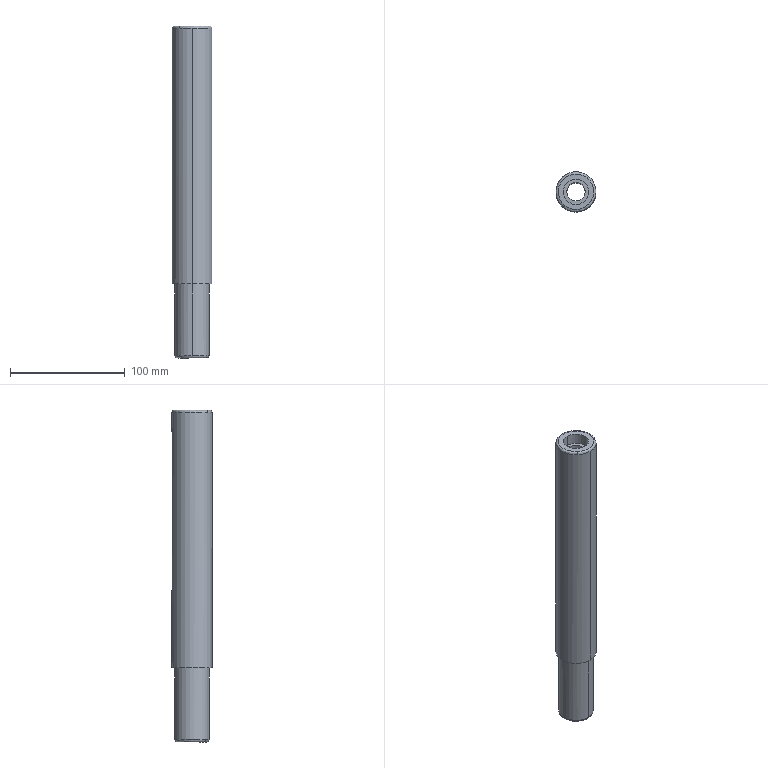Part | SolidWorks | features BaseBody 1 | 1 solid | 35 faces | box 35 x 35 x 289.662 mm | volume 200187 mm3 | cylinder 16 | cone 8 | plane 7 | spline 4 | commonest cylinder face diameters 2.05 x4 4 x2 16 x2 17 x2 22 x2 30 x2
STEP:
#1=CARTESIAN_POINT('',(579.381,24.865,244.432));
#2=VERTEX_POINT('',#1);
#3=CARTESIAN_POINT('',(590.535,55.849,244.432));
#4=VERTEX_POINT('',#3);
#5=CARTESIAN_POINT('',(590.535,38.349,244.432));
#6=DIRECTION('',(0.,0.,-1.));
#7=DIRECTION('',(0.,1.,0.));
#8=AXIS2_PLACEMENT_3D('',#5,#6,#7);
#9=CIRCLE('',#8,17.5);
#10=EDGE_CURVE('',#2,#4,#9,.T.);
#11=ORIENTED_EDGE('',*,*,#10,.F.);
#12=CARTESIAN_POINT('',(580.656,26.406,246.432));
#13=VERTEX_POINT('',#12);
#14=CARTESIAN_POINT('',(580.656,26.406,244.432));
#15=DIRECTION('',(-0.7706,0.6374,0.));
#16=DIRECTION('',(-0.6374,-0.7706,0.));
#17=AXIS2_PLACEMENT_3D('',#14,#15,#16);
#18=CIRCLE('',#17,2.);
#19=EDGE_CURVE('',#2,#13,#18,.T.);
#20=ORIENTED_EDGE('',*,*,#19,.T.);
#21=CARTESIAN_POINT('',(600.414,50.293,246.432));
#22=VERTEX_POINT('',#21);
#23=CARTESIAN_POINT('',(580.656,26.406,246.432));
#24=CARTESIAN_POINT('',(556.769,46.164,246.432));
#25=CARTESIAN_POINT('',(576.527,70.051,246.432));
#26=CARTESIAN_POINT('',(600.414,50.293,246.432));
#27=(BOUNDED_CURVE()B_SPLINE_CURVE(3,(#23,#24,#25,#26),.UNSPECIFIED.,.F.,.F.)B_SPLINE_CURVE_WITH_KNOTS((4,4),(0.,1.),.UNSPECIFIED.)CURVE()GEOMETRIC_REPRESENTATION_ITEM()RATIONAL_B_SPLINE_CURVE((1.,0.3333,0.3333,1.))REPRESENTATION_ITEM(''));
#28=EDGE_CURVE('',#13,#22,#27,.T.);
#29=ORIENTED_EDGE('',*,*,#28,.T.);
#30=CARTESIAN_POINT('',(601.689,51.834,244.432));
#31=VERTEX_POINT('',#30);
#32=CARTESIAN_POINT('',(600.414,50.293,244.432));
#33=DIRECTION('',(0.7706,-0.6374,0.));
#34=DIRECTION('',(0.6374,0.7706,0.));
#35=AXIS2_PLACEMENT_3D('',#32,#33,#34);
#36=CIRCLE('',#35,2.);
#37=EDGE_CURVE('',#31,#22,#36,.T.);
#38=ORIENTED_EDGE('',*,*,#37,.F.);
#39=CARTESIAN_POINT('',(590.535,38.349,244.432));
#40=DIRECTION('',(0.,0.,-1.));
#41=DIRECTION('',(0.,1.,0.));
#42=AXIS2_PLACEMENT_3D('',#39,#40,#41);
#43=CIRCLE('',#42,17.5);
#44=EDGE_CURVE('',#4,#31,#43,.T.);
#45=ORIENTED_EDGE('',*,*,#44,.F.);
#46=EDGE_LOOP('',(#11,#20,#29,#38,#45));
#47=FACE_OUTER_BOUND('',#46,.T.);
#48=CARTESIAN_POINT('',(579.381,24.865,244.432));
#49=CARTESIAN_POINT('',(552.412,47.172,244.432));
#50=CARTESIAN_POINT('',(574.719,74.142,244.432));
#51=CARTESIAN_POINT('',(601.689,51.834,244.432));
#52=CARTESIAN_POINT('',(579.381,24.865,245.604));
#53=CARTESIAN_POINT('',(552.412,47.172,245.604));
#54=CARTESIAN_POINT('',(574.719,74.142,245.604));
#55=CARTESIAN_POINT('',(601.689,51.834,245.604));
#56=CARTESIAN_POINT('',(579.909,25.503,246.432));
#57=CARTESIAN_POINT('',(554.216,46.755,246.432));
#58=CARTESIAN_POINT('',(575.468,72.448,246.432));
#59=CARTESIAN_POINT('',(601.161,51.196,246.432));
#60=CARTESIAN_POINT('',(580.656,26.406,246.432));
#61=CARTESIAN_POINT('',(556.769,46.164,246.432));
#62=CARTESIAN_POINT('',(576.527,70.051,246.432));
#63=CARTESIAN_POINT('',(600.414,50.293,246.432));
#64=(BOUNDED_SURFACE()B_SPLINE_SURFACE(3,3,((#48,#49,#50,#51),(#52,#53,#54,#55),(#56,#57,#58,#59),(#60,#61,#62,#63)),.UNSPECIFIED.,.F.,.F.,.F.)B_SPLINE_SURFACE_WITH_KNOTS((4,4),(4,4),(0.,1.),(0.,1.),.UNSPECIFIED.)GEOMETRIC_REPRESENTATION_ITEM()RATIONAL_B_SPLINE_SURFACE(((1.,0.3333,0.3333,1.),(0.8047,0.2682,0.2682,0.8047),(0.8047,0.2682,0.2682,0.8047),(1.,0.3333,0.3333,1.)))REPRESENTATION_ITEM('')SURFACE());
#65=ADVANCED_FACE('',(#47),#64,.T.);
#66=CARTESIAN_POINT('',(580.975,26.791,-41.23));
#67=VERTEX_POINT('',#66);
#68=CARTESIAN_POINT('',(590.535,23.349,-41.23));
#69=VERTEX_POINT('',#68);
#70=CARTESIAN_POINT('',(590.535,38.349,-41.23));
#71=DIRECTION('',(0.,0.,1.));
#72=DIRECTION('',(0.,1.,0.));
#73=AXIS2_PLACEMENT_3D('',#70,#71,#72);
#74=CIRCLE('',#73,15.);
#75=EDGE_CURVE('',#67,#69,#74,.T.);
#76=ORIENTED_EDGE('',*,*,#75,.F.);
#77=CARTESIAN_POINT('',(582.249,28.332,-43.23));
#78=VERTEX_POINT('',#77);
#79=CARTESIAN_POINT('',(582.249,28.332,-41.23));
#80=DIRECTION('',(0.7706,-0.6374,0.));
#81=DIRECTION('',(-0.6374,-0.7706,0.));
#82=AXIS2_PLACEMENT_3D('',#79,#80,#81);
#83=CIRCLE('',#82,2.);
#84=EDGE_CURVE('',#67,#78,#83,.T.);
#85=ORIENTED_EDGE('',*,*,#84,.T.);
#86=CARTESIAN_POINT('',(598.821,48.367,-43.23));
#87=VERTEX_POINT('',#86);
#88=CARTESIAN_POINT('',(582.249,28.332,-43.23));
#89=CARTESIAN_POINT('',(602.284,11.761,-43.23));
#90=CARTESIAN_POINT('',(618.856,31.795,-43.23));
#91=CARTESIAN_POINT('',(598.821,48.367,-43.23));
#92=(BOUNDED_CURVE()B_SPLINE_CURVE(3,(#88,#89,#90,#91),.UNSPECIFIED.,.F.,.T.)B_SPLINE_CURVE_WITH_KNOTS((4,4),(0.,1.),.UNSPECIFIED.)CURVE()GEOMETRIC_REPRESENTATION_ITEM()RATIONAL_B_SPLINE_CURVE((1.,0.3333,0.3333,1.))REPRESENTATION_ITEM(''));
#93=EDGE_CURVE('',#78,#87,#92,.T.);
#94=ORIENTED_EDGE('',*,*,#93,.T.);
#95=CARTESIAN_POINT('',(600.096,49.908,-41.23));
#96=VERTEX_POINT('',#95);
#97=CARTESIAN_POINT('',(598.821,48.367,-41.23));
#98=DIRECTION('',(-0.7706,0.6374,0.));
#99=DIRECTION('',(0.6374,0.7706,0.));
#100=AXIS2_PLACEMENT_3D('',#97,#98,#99);
#101=CIRCLE('',#100,2.);
#102=EDGE_CURVE('',#96,#87,#101,.T.);
#103=ORIENTED_EDGE('',*,*,#102,.F.);
#104=CARTESIAN_POINT('',(590.535,38.349,-41.23));
#105=DIRECTION('',(0.,0.,1.));
#106=DIRECTION('',(0.,1.,0.));
#107=AXIS2_PLACEMENT_3D('',#104,#105,#106);
#108=CIRCLE('',#107,15.);
#109=EDGE_CURVE('',#69,#96,#108,.T.);
#110=ORIENTED_EDGE('',*,*,#109,.F.);
#111=EDGE_LOOP('',(#76,#85,#94,#103,#110));
#112=FACE_OUTER_BOUND('',#111,.T.);
#113=CARTESIAN_POINT('',(580.975,26.791,-41.23));
#114=CARTESIAN_POINT('',(604.092,7.67,-41.23));
#115=CARTESIAN_POINT('',(623.212,30.787,-41.23));
#116=CARTESIAN_POINT('',(600.096,49.908,-41.23));
#117=CARTESIAN_POINT('',(580.975,26.791,-42.401));
#118=CARTESIAN_POINT('',(604.092,7.67,-42.401));
#119=CARTESIAN_POINT('',(623.212,30.787,-42.401));
#120=CARTESIAN_POINT('',(600.096,49.908,-42.401));
#121=CARTESIAN_POINT('',(581.503,27.429,-43.23));
#122=CARTESIAN_POINT('',(603.343,9.364,-43.23));
#123=CARTESIAN_POINT('',(621.408,31.205,-43.23));
#124=CARTESIAN_POINT('',(599.568,49.27,-43.23));
#125=CARTESIAN_POINT('',(582.249,28.332,-43.23));
#126=CARTESIAN_POINT('',(602.284,11.761,-43.23));
#127=CARTESIAN_POINT('',(618.856,31.795,-43.23));
#128=CARTESIAN_POINT('',(598.821,48.367,-43.23));
#129=(BOUNDED_SURFACE()B_SPLINE_SURFACE(3,3,((#113,#114,#115,#116),(#117,#118,#119,#120),(#121,#122,#123,#124),(#125,#126,#127,#128)),.UNSPECIFIED.,.F.,.F.,.F.)B_SPLINE_SURFACE_WITH_KNOTS((4,4),(4,4),(0.,1.),(0.,1.),.UNSPECIFIED.)GEOMETRIC_REPRESENTATION_ITEM()RATIONAL_B_SPLINE_SURFACE(((1.,0.3333,0.3333,1.),(0.8047,0.2682,0.2682,0.8047),(0.8047,0.2682,0.2682,0.8047),(1.,0.3333,0.3333,1.)))REPRESENTATION_ITEM('')SURFACE());
#130=ADVANCED_FACE('',(#112),#129,.T.);
#131=ORIENTED_EDGE('',*,*,#44,.T.);
#132=CARTESIAN_POINT('',(590.535,20.849,244.432));
#133=VERTEX_POINT('',#132);
#134=CARTESIAN_POINT('',(590.535,38.349,244.432));
#135=DIRECTION('',(0.,0.,-1.));
#136=DIRECTION('',(0.,1.,0.));
#137=AXIS2_PLACEMENT_3D('',#134,#135,#136);
#138=CIRCLE('',#137,17.5);
#139=EDGE_CURVE('',#31,#133,#138,.T.);
#140=ORIENTED_EDGE('',*,*,#139,.T.);
#141=CARTESIAN_POINT('',(590.535,20.849,21.432));
#142=VERTEX_POINT('',#141);
#143=CARTESIAN_POINT('',(590.535,20.849,246.432));
#144=DIRECTION('',(0.,0.,-1.));
#145=VECTOR('',#144,1000.);
#146=LINE('',#143,#145);
#147=EDGE_CURVE('',#133,#142,#146,.T.);
#148=ORIENTED_EDGE('',*,*,#147,.T.);
#149=CARTESIAN_POINT('',(590.535,55.849,21.432));
#150=VERTEX_POINT('',#149);
#151=CARTESIAN_POINT('',(590.535,38.349,21.432));
#152=DIRECTION('',(0.,0.,1.));
#153=DIRECTION('',(0.,1.,0.));
#154=AXIS2_PLACEMENT_3D('',#151,#152,#153);
#155=CIRCLE('',#154,17.5);
#156=EDGE_CURVE('',#142,#150,#155,.T.);
#157=ORIENTED_EDGE('',*,*,#156,.T.);
#158=CARTESIAN_POINT('',(590.535,55.849,88.433));
#159=VERTEX_POINT('',#158);
#160=CARTESIAN_POINT('',(590.535,55.849,246.432));
#161=DIRECTION('',(0.,0.,-1.));
#162=VECTOR('',#161,1000.);
#163=LINE('',#160,#162);
#164=EDGE_CURVE('',#159,#150,#163,.T.);
#165=ORIENTED_EDGE('',*,*,#164,.F.);
#166=CARTESIAN_POINT('',(592.459,55.743,90.432));
#167=VERTEX_POINT('',#166);
#168=CARTESIAN_POINT('',(590.535,55.849,88.433));
#169=CARTESIAN_POINT('',(590.663,55.849,88.438));
#170=CARTESIAN_POINT('',(590.789,55.848,88.455));
#171=CARTESIAN_POINT('',(591.037,55.843,88.513));
#172=CARTESIAN_POINT('',(591.161,55.839,88.555));
#173=CARTESIAN_POINT('',(591.393,55.829,88.659));
#174=CARTESIAN_POINT('',(591.504,55.823,88.722));
#175=CARTESIAN_POINT('',(591.713,55.81,88.868));
#176=CARTESIAN_POINT('',(591.811,55.803,88.953));
#177=CARTESIAN_POINT('',(592.076,55.782,89.227));
#178=CARTESIAN_POINT('',(592.218,55.769,89.446));
#179=CARTESIAN_POINT('',(592.409,55.749,89.918));
#180=CARTESIAN_POINT('',(592.459,55.743,90.174));
#181=CARTESIAN_POINT('',(592.459,55.743,90.432));
#182=B_SPLINE_CURVE_WITH_KNOTS('',3,(#168,#169,#170,#171,#172,#173,#174,#175,#176,#177,#178,#179,#180,#181),.UNSPECIFIED.,.F.,.F.,(4,2,2,2,2,2,4),(0.00007532,0.0004568,0.0008382,0.00122,0.001601,0.002364,0.003127),.UNSPECIFIED.);
#183=EDGE_CURVE('',#159,#167,#182,.T.);
#184=ORIENTED_EDGE('',*,*,#183,.T.);
#185=CARTESIAN_POINT('',(592.459,55.743,226.432));
#186=VERTEX_POINT('',#185);
#187=CARTESIAN_POINT('',(592.459,55.743,246.432));
#188=DIRECTION('',(0.,0.,1.));
#189=VECTOR('',#188,1000.);
#190=LINE('',#187,#189);
#191=EDGE_CURVE('',#167,#186,#190,.T.);
#192=ORIENTED_EDGE('',*,*,#191,.T.);
#193=CARTESIAN_POINT('',(590.535,55.849,228.431));
#194=VERTEX_POINT('',#193);
#195=CARTESIAN_POINT('',(592.459,55.743,226.432));
#196=CARTESIAN_POINT('',(592.459,55.743,226.561));
#197=CARTESIAN_POINT('',(592.447,55.745,226.688));
#198=CARTESIAN_POINT('',(592.399,55.75,226.937));
#199=CARTESIAN_POINT('',(592.362,55.754,227.061));
#200=CARTESIAN_POINT('',(592.266,55.764,227.299));
#201=CARTESIAN_POINT('',(592.208,55.769,227.412));
#202=CARTESIAN_POINT('',(592.069,55.782,227.625));
#203=CARTESIAN_POINT('',(591.989,55.789,227.727));
#204=CARTESIAN_POINT('',(591.812,55.803,227.911));
#205=CARTESIAN_POINT('',(591.716,55.81,227.993));
#206=CARTESIAN_POINT('',(591.507,55.823,228.141));
#207=CARTESIAN_POINT('',(591.394,55.829,228.204));
#208=CARTESIAN_POINT('',(591.046,55.844,228.361));
#209=CARTESIAN_POINT('',(590.792,55.849,228.421));
#210=CARTESIAN_POINT('',(590.535,55.849,228.431));
#211=B_SPLINE_CURVE_WITH_KNOTS('',3,(#195,#196,#197,#198,#199,#200,#201,#202,#203,#204,#205,#206,#207,#208,#209,#210),.UNSPECIFIED.,.F.,.F.,(4,2,2,2,2,2,2,4),(-0.003127,-0.002745,-0.002364,-0.001982,-0.001601,-0.00122,-0.0008381,-0.00007524),.UNSPECIFIED.);
#212=EDGE_CURVE('',#186,#194,#211,.T.);
#213=ORIENTED_EDGE('',*,*,#212,.T.);
#214=CARTESIAN_POINT('',(590.535,55.849,246.432));
#215=DIRECTION('',(0.,0.,-1.));
#216=VECTOR('',#215,1000.);
#217=LINE('',#214,#216);
#218=EDGE_CURVE('',#4,#194,#217,.T.);
#219=ORIENTED_EDGE('',*,*,#218,.F.);
#220=EDGE_LOOP('',(#131,#140,#148,#157,#165,#184,#192,#213,#219));
#221=FACE_OUTER_BOUND('',#220,.T.);
#222=CARTESIAN_POINT('',(590.535,38.349,246.432));
#223=DIRECTION('',(0.,0.,-1.));
#224=DIRECTION('',(0.,1.,0.));
#225=AXIS2_PLACEMENT_3D('',#222,#223,#224);
#226=CYLINDRICAL_SURFACE('',#225,17.5);
#227=ADVANCED_FACE('',(#221),#226,.T.);
#228=CARTESIAN_POINT('',(590.535,23.349,21.432));
#229=VERTEX_POINT('',#228);
#230=CARTESIAN_POINT('',(590.535,53.349,21.432));
#231=VERTEX_POINT('',#230);
#232=CARTESIAN_POINT('',(590.535,38.349,21.432));
#233=DIRECTION('',(0.,0.,1.));
#234=DIRECTION('',(0.,1.,0.));
#235=AXIS2_PLACEMENT_3D('',#232,#233,#234);
#236=CIRCLE('',#235,15.);
#237=EDGE_CURVE('',#229,#231,#236,.T.);
#238=ORIENTED_EDGE('',*,*,#237,.F.);
#239=CARTESIAN_POINT('',(590.535,23.349,21.432));
#240=DIRECTION('',(0.,0.,-1.));
#241=VECTOR('',#240,1000.);
#242=LINE('',#239,#241);
#243=EDGE_CURVE('',#229,#69,#242,.T.);
#244=ORIENTED_EDGE('',*,*,#243,.T.);
#245=ORIENTED_EDGE('',*,*,#109,.T.);
#246=CARTESIAN_POINT('',(590.535,53.349,-41.23));
#247=VERTEX_POINT('',#246);
#248=CARTESIAN_POINT('',(590.535,38.349,-41.23));
#249=DIRECTION('',(0.,0.,1.));
#250=DIRECTION('',(0.,1.,0.));
#251=AXIS2_PLACEMENT_3D('',#248,#249,#250);
#252=CIRCLE('',#251,15.);
#253=EDGE_CURVE('',#96,#247,#252,.T.);
#254=ORIENTED_EDGE('',*,*,#253,.T.);
#255=CARTESIAN_POINT('',(590.535,53.349,21.432));
#256=DIRECTION('',(0.,0.,-1.));
#257=VECTOR('',#256,1000.);
#258=LINE('',#255,#257);
#259=EDGE_CURVE('',#231,#247,#258,.T.);
#260=ORIENTED_EDGE('',*,*,#259,.F.);
#261=EDGE_LOOP('',(#238,#244,#245,#254,#260));
#262=FACE_OUTER_BOUND('',#261,.T.);
#263=CARTESIAN_POINT('',(590.535,38.349,21.432));
#264=DIRECTION('',(0.,0.,-1.));
#265=DIRECTION('',(0.,1.,0.));
#266=AXIS2_PLACEMENT_3D('',#263,#264,#265);
#267=CYLINDRICAL_SURFACE('',#266,15.);
#268=ADVANCED_FACE('',(#262),#267,.T.);
#269=CARTESIAN_POINT('',(590.535,49.349,246.432));
#270=VERTEX_POINT('',#269);
#271=CARTESIAN_POINT('',(590.535,27.349,246.432));
#272=VERTEX_POINT('',#271);
#273=CARTESIAN_POINT('',(590.535,38.349,246.432));
#274=DIRECTION('',(0.,0.,1.));
#275=DIRECTION('',(0.,1.,0.));
#276=AXIS2_PLACEMENT_3D('',#273,#274,#275);
#277=CIRCLE('',#276,11.);
#278=EDGE_CURVE('',#270,#272,#277,.T.);
#279=ORIENTED_EDGE('',*,*,#278,.T.);
#280=CARTESIAN_POINT('',(590.535,27.349,236.432));
#281=VERTEX_POINT('',#280);
#282=CARTESIAN_POINT('',(590.535,27.349,246.432));
#283=DIRECTION('',(0.,0.,-1.));
#284=VECTOR('',#283,1000.);
#285=LINE('',#282,#284);
#286=EDGE_CURVE('',#272,#281,#285,.T.);
#287=ORIENTED_EDGE('',*,*,#286,.T.);
#288=CARTESIAN_POINT('',(590.535,49.349,236.432));
#289=VERTEX_POINT('',#288);
#290=CARTESIAN_POINT('',(590.535,38.349,236.432));
#291=DIRECTION('',(0.,0.,1.));
#292=DIRECTION('',(0.,1.,0.));
#293=AXIS2_PLACEMENT_3D('',#290,#291,#292);
#294=CIRCLE('',#293,11.);
#295=EDGE_CURVE('',#289,#281,#294,.T.);
#296=ORIENTED_EDGE('',*,*,#295,.F.);
#297=CARTESIAN_POINT('',(590.535,49.349,246.432));
#298=DIRECTION('',(0.,0.,-1.));
#299=VECTOR('',#298,1000.);
#300=LINE('',#297,#299);
#301=EDGE_CURVE('',#270,#289,#300,.T.);
#302=ORIENTED_EDGE('',*,*,#301,.F.);
#303=EDGE_LOOP('',(#279,#287,#296,#302));
#304=FACE_OUTER_BOUND('',#303,.T.);
#305=CARTESIAN_POINT('',(590.535,38.349,246.432));
#306=DIRECTION('',(0.,0.,-1.));
#307=DIRECTION('',(0.,1.,0.));
#308=AXIS2_PLACEMENT_3D('',#305,#306,#307);
#309=CYLINDRICAL_SURFACE('',#308,11.);
#310=ADVANCED_FACE('',(#304),#309,.F.);
#311=CARTESIAN_POINT('',(591.494,53.654,226.432));
#312=VERTEX_POINT('',#311);
#313=CARTESIAN_POINT('',(589.444,53.645,226.432));
#314=VERTEX_POINT('',#313);
#315=CARTESIAN_POINT('',(590.469,53.649,226.432));
#316=DIRECTION('',(-0.004352,1.,0.));
#317=DIRECTION('',(-1.,-0.004352,0.));
#318=AXIS2_PLACEMENT_3D('',#315,#316,#317);
#319=CIRCLE('',#318,1.025);
#320=EDGE_CURVE('',#312,#314,#319,.T.);
#321=ORIENTED_EDGE('',*,*,#320,.F.);
#322=CARTESIAN_POINT('',(591.693,53.855,226.432));
#323=VERTEX_POINT('',#322);
#324=CARTESIAN_POINT('',(591.693,53.855,226.432));
#325=DIRECTION('',(0.704,0.7102,0.));
#326=VECTOR('',#325,1000.);
#327=LINE('',#324,#326);
#328=EDGE_CURVE('',#312,#323,#327,.T.);
#329=ORIENTED_EDGE('',*,*,#328,.T.);
#330=CARTESIAN_POINT('',(589.243,53.844,226.432));
#331=VERTEX_POINT('',#330);
#332=CARTESIAN_POINT('',(590.468,53.849,226.432));
#333=DIRECTION('',(-0.004352,1.,0.));
#334=DIRECTION('',(-1.,-0.004352,0.));
#335=AXIS2_PLACEMENT_3D('',#332,#333,#334);
#336=CIRCLE('',#335,1.225);
#337=EDGE_CURVE('',#323,#331,#336,.T.);
#338=ORIENTED_EDGE('',*,*,#337,.T.);
#339=CARTESIAN_POINT('',(589.243,53.844,226.432));
#340=DIRECTION('',(-0.7102,0.704,0.));
#341=VECTOR('',#340,1000.);
#342=LINE('',#339,#341);
#343=EDGE_CURVE('',#314,#331,#342,.T.);
#344=ORIENTED_EDGE('',*,*,#343,.F.);
#345=EDGE_LOOP('',(#321,#329,#338,#344));
#346=FACE_OUTER_BOUND('',#345,.T.);
#347=CARTESIAN_POINT('',(590.468,53.849,226.432));
#348=DIRECTION('',(-0.004352,1.,0.));
#349=DIRECTION('',(-1.,-0.004352,0.));
#350=AXIS2_PLACEMENT_3D('',#347,#348,#349);
#351=CONICAL_SURFACE('',#350,1.225,0.7854);
#352=ADVANCED_FACE('',(#346),#351,.F.);
#353=CARTESIAN_POINT('',(591.494,53.654,90.432));
#354=VERTEX_POINT('',#353);
#355=CARTESIAN_POINT('',(589.444,53.645,90.432));
#356=VERTEX_POINT('',#355);
#357=CARTESIAN_POINT('',(590.469,53.649,90.432));
#358=DIRECTION('',(-0.004352,1.,0.));
#359=DIRECTION('',(-1.,-0.004352,0.));
#360=AXIS2_PLACEMENT_3D('',#357,#358,#359);
#361=CIRCLE('',#360,1.025);
#362=EDGE_CURVE('',#354,#356,#361,.T.);
#363=ORIENTED_EDGE('',*,*,#362,.F.);
#364=CARTESIAN_POINT('',(591.693,53.855,90.432));
#365=VERTEX_POINT('',#364);
#366=CARTESIAN_POINT('',(591.693,53.855,90.432));
#367=DIRECTION('',(0.704,0.7102,0.));
#368=VECTOR('',#367,1000.);
#369=LINE('',#366,#368);
#370=EDGE_CURVE('',#354,#365,#369,.T.);
#371=ORIENTED_EDGE('',*,*,#370,.T.);
#372=CARTESIAN_POINT('',(589.243,53.844,90.432));
#373=VERTEX_POINT('',#372);
#374=CARTESIAN_POINT('',(590.468,53.849,90.432));
#375=DIRECTION('',(-0.004352,1.,0.));
#376=DIRECTION('',(-1.,-0.004352,0.));
#377=AXIS2_PLACEMENT_3D('',#374,#375,#376);
#378=CIRCLE('',#377,1.225);
#379=EDGE_CURVE('',#365,#373,#378,.T.);
#380=ORIENTED_EDGE('',*,*,#379,.T.);
#381=CARTESIAN_POINT('',(589.243,53.844,90.432));
#382=DIRECTION('',(-0.7102,0.704,0.));
#383=VECTOR('',#382,1000.);
#384=LINE('',#381,#383);
#385=EDGE_CURVE('',#356,#373,#384,.T.);
#386=ORIENTED_EDGE('',*,*,#385,.F.);
#387=EDGE_LOOP('',(#363,#371,#380,#386));
#388=FACE_OUTER_BOUND('',#387,.T.);
#389=CARTESIAN_POINT('',(590.468,53.849,90.432));
#390=DIRECTION('',(-0.004352,1.,0.));
#391=DIRECTION('',(-1.,-0.004352,0.));
#392=AXIS2_PLACEMENT_3D('',#389,#390,#391);
#393=CONICAL_SURFACE('',#392,1.225,0.7854);
#394=ADVANCED_FACE('',(#388),#393,.F.);
#395=CARTESIAN_POINT('',(590.535,46.349,-17.734));
#396=VERTEX_POINT('',#395);
#397=CARTESIAN_POINT('',(590.535,30.349,-17.734));
#398=VERTEX_POINT('',#397);
#399=CARTESIAN_POINT('',(590.535,38.349,-17.734));
#400=DIRECTION('',(0.,0.,1.));
#401=DIRECTION('',(0.,-1.,0.));
#402=AXIS2_PLACEMENT_3D('',#399,#400,#401);
#403=CIRCLE('',#402,8.);
#404=EDGE_CURVE('',#396,#398,#403,.T.);
#405=ORIENTED_EDGE('',*,*,#404,.F.);
#406=CARTESIAN_POINT('',(590.535,46.349,89.408));
#407=VERTEX_POINT('',#406);
#408=CARTESIAN_POINT('',(590.535,46.349,-43.568));
#409=DIRECTION('',(0.,0.,1.));
#410=VECTOR('',#409,1000.);
#411=LINE('',#408,#410);
#412=EDGE_CURVE('',#396,#407,#411,.T.);
#413=ORIENTED_EDGE('',*,*,#412,.T.);
#414=CARTESIAN_POINT('',(589.476,46.279,90.432));
#415=VERTEX_POINT('',#414);
#416=CARTESIAN_POINT('',(589.476,46.279,90.432));
#417=CARTESIAN_POINT('',(589.476,46.279,90.293));
#418=CARTESIAN_POINT('',(589.504,46.283,90.157));
#419=CARTESIAN_POINT('',(589.611,46.296,89.905));
#420=CARTESIAN_POINT('',(589.69,46.305,89.79));
#421=CARTESIAN_POINT('',(589.886,46.324,89.6));
#422=CARTESIAN_POINT('',(590.005,46.333,89.524));
#423=CARTESIAN_POINT('',(590.26,46.346,89.426));
#424=CARTESIAN_POINT('',(590.398,46.349,89.403));
#425=CARTESIAN_POINT('',(590.535,46.349,89.408));
#426=B_SPLINE_CURVE_WITH_KNOTS('',3,(#416,#417,#418,#419,#420,#421,#422,#423,#424,#425),.UNSPECIFIED.,.F.,.F.,(4,2,2,2,4),(0.,0.0004098,0.0008195,0.001229,0.001639),.UNSPECIFIED.);
#427=EDGE_CURVE('',#415,#407,#426,.T.);
#428=ORIENTED_EDGE('',*,*,#427,.F.);
#429=CARTESIAN_POINT('',(590.535,46.349,91.456));
#430=VERTEX_POINT('',#429);
#431=CARTESIAN_POINT('',(590.535,46.349,91.456));
#432=CARTESIAN_POINT('',(590.399,46.349,91.461));
#433=CARTESIAN_POINT('',(590.26,46.346,91.438));
#434=CARTESIAN_POINT('',(590.005,46.333,91.34));
#435=CARTESIAN_POINT('',(589.888,46.324,91.265));
#436=CARTESIAN_POINT('',(589.59,46.296,90.978));
#437=CARTESIAN_POINT('',(589.476,46.279,90.709));
#438=CARTESIAN_POINT('',(589.476,46.279,90.432));
#439=B_SPLINE_CURVE_WITH_KNOTS('',3,(#431,#432,#433,#434,#435,#436,#437,#438),.UNSPECIFIED.,.F.,.F.,(4,2,2,4),(0.004777,0.005186,0.005596,0.006414),.UNSPECIFIED.);
#440=EDGE_CURVE('',#430,#415,#439,.T.);
#441=ORIENTED_EDGE('',*,*,#440,.F.);
#442=CARTESIAN_POINT('',(590.535,46.349,225.408));
#443=VERTEX_POINT('',#442);
#444=CARTESIAN_POINT('',(590.535,46.349,-43.568));
#445=DIRECTION('',(0.,0.,1.));
#446=VECTOR('',#445,1000.);
#447=LINE('',#444,#446);
#448=EDGE_CURVE('',#430,#443,#447,.T.);
#449=ORIENTED_EDGE('',*,*,#448,.T.);
#450=CARTESIAN_POINT('',(589.476,46.279,226.432));
#451=VERTEX_POINT('',#450);
#452=CARTESIAN_POINT('',(589.476,46.279,226.432));
#453=CARTESIAN_POINT('',(589.476,46.279,226.293));
#454=CARTESIAN_POINT('',(589.504,46.283,226.157));
#455=CARTESIAN_POINT('',(589.611,46.296,225.905));
#456=CARTESIAN_POINT('',(589.69,46.305,225.79));
#457=CARTESIAN_POINT('',(589.886,46.324,225.6));
#458=CARTESIAN_POINT('',(590.005,46.333,225.524));
#459=CARTESIAN_POINT('',(590.26,46.346,225.426));
#460=CARTESIAN_POINT('',(590.398,46.349,225.403));
#461=CARTESIAN_POINT('',(590.535,46.349,225.408));
#462=B_SPLINE_CURVE_WITH_KNOTS('',3,(#452,#453,#454,#455,#456,#457,#458,#459,#460,#461),.UNSPECIFIED.,.F.,.F.,(4,2,2,2,4),(0.,0.0004098,0.0008195,0.001229,0.001639),.UNSPECIFIED.);
#463=EDGE_CURVE('',#451,#443,#462,.T.);
#464=ORIENTED_EDGE('',*,*,#463,.F.);
#465=CARTESIAN_POINT('',(590.535,46.349,227.456));
#466=VERTEX_POINT('',#465);
#467=CARTESIAN_POINT('',(590.535,46.349,227.456));
#468=CARTESIAN_POINT('',(590.399,46.349,227.461));
#469=CARTESIAN_POINT('',(590.26,46.346,227.438));
#470=CARTESIAN_POINT('',(590.005,46.333,227.34));
#471=CARTESIAN_POINT('',(589.888,46.324,227.265));
#472=CARTESIAN_POINT('',(589.59,46.296,226.978));
#473=CARTESIAN_POINT('',(589.476,46.279,226.709));
#474=CARTESIAN_POINT('',(589.476,46.279,226.432));
#475=B_SPLINE_CURVE_WITH_KNOTS('',3,(#467,#468,#469,#470,#471,#472,#473,#474),.UNSPECIFIED.,.F.,.F.,(4,2,2,4),(0.004777,0.005186,0.005596,0.006414),.UNSPECIFIED.);
#476=EDGE_CURVE('',#466,#451,#475,.T.);
#477=ORIENTED_EDGE('',*,*,#476,.F.);
#478=CARTESIAN_POINT('',(590.535,46.349,236.432));
#479=VERTEX_POINT('',#478);
#480=CARTESIAN_POINT('',(590.535,46.349,-43.568));
#481=DIRECTION('',(0.,0.,1.));
#482=VECTOR('',#481,1000.);
#483=LINE('',#480,#482);
#484=EDGE_CURVE('',#466,#479,#483,.T.);
#485=ORIENTED_EDGE('',*,*,#484,.T.);
#486=CARTESIAN_POINT('',(590.535,30.349,236.432));
#487=VERTEX_POINT('',#486);
#488=CARTESIAN_POINT('',(590.535,38.349,236.432));
#489=DIRECTION('',(0.,0.,1.));
#490=DIRECTION('',(0.,-1.,0.));
#491=AXIS2_PLACEMENT_3D('',#488,#489,#490);
#492=CIRCLE('',#491,8.);
#493=EDGE_CURVE('',#479,#487,#492,.T.);
#494=ORIENTED_EDGE('',*,*,#493,.T.);
#495=CARTESIAN_POINT('',(590.535,30.349,-43.568));
#496=DIRECTION('',(0.,0.,1.));
#497=VECTOR('',#496,1000.);
#498=LINE('',#495,#497);
#499=EDGE_CURVE('',#398,#487,#498,.T.);
#500=ORIENTED_EDGE('',*,*,#499,.F.);
#501=EDGE_LOOP('',(#405,#413,#428,#441,#449,#464,#477,#485,#494,#500));
#502=FACE_OUTER_BOUND('',#501,.T.);
#503=CARTESIAN_POINT('',(590.535,38.349,-43.568));
#504=DIRECTION('',(0.,0.,1.));
#505=DIRECTION('',(0.,-1.,0.));
#506=AXIS2_PLACEMENT_3D('',#503,#504,#505);
#507=CYLINDRICAL_SURFACE('',#506,8.);
#508=ADVANCED_FACE('',(#502),#507,.F.);
#509=ORIENTED_EDGE('',*,*,#320,.T.);
#510=CARTESIAN_POINT('',(589.46,49.845,226.432));
#511=DIRECTION('',(0.004352,-1.,0.));
#512=VECTOR('',#511,1000.);
#513=LINE('',#510,#512);
#514=EDGE_CURVE('',#314,#451,#513,.T.);
#515=ORIENTED_EDGE('',*,*,#514,.T.);
#516=ORIENTED_EDGE('',*,*,#463,.T.);
#517=CARTESIAN_POINT('',(591.526,46.288,226.432));
#518=VERTEX_POINT('',#517);
#519=CARTESIAN_POINT('',(590.535,46.349,225.408));
#520=CARTESIAN_POINT('',(590.666,46.349,225.412));
#521=CARTESIAN_POINT('',(590.796,46.346,225.442));
#522=CARTESIAN_POINT('',(591.037,46.335,225.549));
#523=CARTESIAN_POINT('',(591.146,46.327,225.625));
#524=CARTESIAN_POINT('',(591.421,46.302,225.909));
#525=CARTESIAN_POINT('',(591.526,46.288,226.167));
#526=CARTESIAN_POINT('',(591.526,46.288,226.432));
#527=B_SPLINE_CURVE_WITH_KNOTS('',3,(#519,#520,#521,#522,#523,#524,#525,#526),.UNSPECIFIED.,.F.,.F.,(4,2,2,4),(0.001639,0.002031,0.002423,0.003207),.UNSPECIFIED.);
#528=EDGE_CURVE('',#443,#518,#527,.T.);
#529=ORIENTED_EDGE('',*,*,#528,.T.);
#530=CARTESIAN_POINT('',(591.51,49.854,226.432));
#531=DIRECTION('',(0.004352,-1.,0.));
#532=VECTOR('',#531,1000.);
#533=LINE('',#530,#532);
#534=EDGE_CURVE('',#312,#518,#533,.T.);
#535=ORIENTED_EDGE('',*,*,#534,.F.);
#536=EDGE_LOOP('',(#509,#515,#516,#529,#535));
#537=FACE_OUTER_BOUND('',#536,.T.);
#538=CARTESIAN_POINT('',(590.485,49.849,226.432));
#539=DIRECTION('',(0.004352,-1.,0.));
#540=DIRECTION('',(1.,0.004352,0.));
#541=AXIS2_PLACEMENT_3D('',#538,#539,#540);
#542=CYLINDRICAL_SURFACE('',#541,1.025);
#543=ADVANCED_FACE('',(#537),#542,.F.);
#544=ORIENTED_EDGE('',*,*,#362,.T.);
#545=CARTESIAN_POINT('',(589.46,49.845,90.432));
#546=DIRECTION('',(0.004352,-1.,0.));
#547=VECTOR('',#546,1000.);
#548=LINE('',#545,#547);
#549=EDGE_CURVE('',#356,#415,#548,.T.);
#550=ORIENTED_EDGE('',*,*,#549,.T.);
#551=ORIENTED_EDGE('',*,*,#427,.T.);
#552=CARTESIAN_POINT('',(591.526,46.288,90.432));
#553=VERTEX_POINT('',#552);
#554=CARTESIAN_POINT('',(590.535,46.349,89.408));
#555=CARTESIAN_POINT('',(590.666,46.349,89.412));
#556=CARTESIAN_POINT('',(590.796,46.346,89.442));
#557=CARTESIAN_POINT('',(591.037,46.335,89.549));
#558=CARTESIAN_POINT('',(591.146,46.327,89.625));
#559=CARTESIAN_POINT('',(591.421,46.302,89.909));
#560=CARTESIAN_POINT('',(591.526,46.288,90.167));
#561=CARTESIAN_POINT('',(591.526,46.288,90.432));
#562=B_SPLINE_CURVE_WITH_KNOTS('',3,(#554,#555,#556,#557,#558,#559,#560,#561),.UNSPECIFIED.,.F.,.F.,(4,2,2,4),(0.001639,0.002031,0.002423,0.003207),.UNSPECIFIED.);
#563=EDGE_CURVE('',#407,#553,#562,.T.);
#564=ORIENTED_EDGE('',*,*,#563,.T.);
#565=CARTESIAN_POINT('',(591.51,49.854,90.432));
#566=DIRECTION('',(0.004352,-1.,0.));
#567=VECTOR('',#566,1000.);
#568=LINE('',#565,#567);
#569=EDGE_CURVE('',#354,#553,#568,.T.);
#570=ORIENTED_EDGE('',*,*,#569,.F.);
#571=EDGE_LOOP('',(#544,#550,#551,#564,#570));
#572=FACE_OUTER_BOUND('',#571,.T.);
#573=CARTESIAN_POINT('',(590.485,49.849,90.432));
#574=DIRECTION('',(0.004352,-1.,0.));
#575=DIRECTION('',(1.,0.004352,0.));
#576=AXIS2_PLACEMENT_3D('',#573,#574,#575);
#577=CYLINDRICAL_SURFACE('',#576,1.025);
#578=ADVANCED_FACE('',(#572),#577,.F.);
#579=CARTESIAN_POINT('',(590.535,46.849,-43.23));
#580=VERTEX_POINT('',#579);
#581=CARTESIAN_POINT('',(590.535,29.849,-43.23));
#582=VERTEX_POINT('',#581);
#583=CARTESIAN_POINT('',(590.535,38.349,-43.23));
#584=DIRECTION('',(0.,0.,1.));
#585=DIRECTION('',(0.,-1.,0.));
#586=AXIS2_PLACEMENT_3D('',#583,#584,#585);
#587=CIRCLE('',#586,8.5);
#588=EDGE_CURVE('',#580,#582,#587,.T.);
#589=ORIENTED_EDGE('',*,*,#588,.F.);
#590=CARTESIAN_POINT('',(590.535,46.849,-23.23));
#591=VERTEX_POINT('',#590);
#592=CARTESIAN_POINT('',(590.535,46.849,-33.23));
#593=DIRECTION('',(0.,0.,1.));
#594=VECTOR('',#593,1000.);
#595=LINE('',#592,#594);
#596=EDGE_CURVE('',#580,#591,#595,.T.);
#597=ORIENTED_EDGE('',*,*,#596,.T.);
#598=CARTESIAN_POINT('',(590.535,29.849,-23.23));
#599=VERTEX_POINT('',#598);
#600=CARTESIAN_POINT('',(590.535,38.349,-23.23));
#601=DIRECTION('',(0.,0.,-1.));
#602=DIRECTION('',(0.,-1.,0.));
#603=AXIS2_PLACEMENT_3D('',#600,#601,#602);
#604=CIRCLE('',#603,8.5);
#605=EDGE_CURVE('',#599,#591,#604,.T.);
#606=ORIENTED_EDGE('',*,*,#605,.F.);
#607=CARTESIAN_POINT('',(590.535,29.849,-33.23));
#608=DIRECTION('',(0.,0.,1.));
#609=VECTOR('',#608,1000.);
#610=LINE('',#607,#609);
#611=EDGE_CURVE('',#582,#599,#610,.T.);
#612=ORIENTED_EDGE('',*,*,#611,.F.);
#613=EDGE_LOOP('',(#589,#597,#606,#612));
#614=FACE_OUTER_BOUND('',#613,.T.);
#615=CARTESIAN_POINT('',(590.535,38.349,-33.23));
#616=DIRECTION('',(0.,0.,1.));
#617=DIRECTION('',(0.,-1.,0.));
#618=AXIS2_PLACEMENT_3D('',#615,#616,#617);
#619=CYLINDRICAL_SURFACE('',#618,8.5);
#620=ADVANCED_FACE('',(#614),#619,.F.);
#621=ORIENTED_EDGE('',*,*,#404,.T.);
#622=CARTESIAN_POINT('',(590.535,29.854,-18.23));
#623=VERTEX_POINT('',#622);
#624=CARTESIAN_POINT('',(590.535,29.854,-18.23));
#625=DIRECTION('',(0.,-0.7069,-0.7073));
#626=VECTOR('',#625,1000.);
#627=LINE('',#624,#626);
#628=EDGE_CURVE('',#398,#623,#627,.T.);
#629=ORIENTED_EDGE('',*,*,#628,.T.);
#630=CARTESIAN_POINT('',(590.535,46.845,-18.23));
#631=VERTEX_POINT('',#630);
#632=CARTESIAN_POINT('',(590.535,38.349,-18.23));
#633=DIRECTION('',(0.,0.,1.));
#634=DIRECTION('',(-0.6374,-0.7706,0.));
#635=AXIS2_PLACEMENT_3D('',#632,#633,#634);
#636=CIRCLE('',#635,8.496);
#637=EDGE_CURVE('',#631,#623,#636,.T.);
#638=ORIENTED_EDGE('',*,*,#637,.F.);
#639=CARTESIAN_POINT('',(590.535,46.845,-18.23));
#640=DIRECTION('',(0.,0.7069,-0.7073));
#641=VECTOR('',#640,1000.);
#642=LINE('',#639,#641);
#643=EDGE_CURVE('',#396,#631,#642,.T.);
#644=ORIENTED_EDGE('',*,*,#643,.F.);
#645=EDGE_LOOP('',(#621,#629,#638,#644));
#646=FACE_OUTER_BOUND('',#645,.T.);
#647=CARTESIAN_POINT('',(590.535,38.349,-18.23));
#648=DIRECTION('',(0.,0.,-1.));
#649=DIRECTION('',(0.,1.,0.));
#650=AXIS2_PLACEMENT_3D('',#647,#648,#649);
#651=CONICAL_SURFACE('',#650,8.496,0.7851);
#652=ADVANCED_FACE('',(#646),#651,.F.);
#653=ORIENTED_EDGE('',*,*,#637,.T.);
#654=CARTESIAN_POINT('',(590.535,29.849,-23.23));
#655=DIRECTION('',(0.,-0.00085,-1.));
#656=VECTOR('',#655,1000.);
#657=LINE('',#654,#656);
#658=EDGE_CURVE('',#623,#599,#657,.T.);
#659=ORIENTED_EDGE('',*,*,#658,.T.);
#660=ORIENTED_EDGE('',*,*,#605,.T.);
#661=CARTESIAN_POINT('',(590.535,46.849,-23.23));
#662=DIRECTION('',(0.,0.00085,-1.));
#663=VECTOR('',#662,1000.);
#664=LINE('',#661,#663);
#665=EDGE_CURVE('',#631,#591,#664,.T.);
#666=ORIENTED_EDGE('',*,*,#665,.F.);
#667=EDGE_LOOP('',(#653,#659,#660,#666));
#668=FACE_OUTER_BOUND('',#667,.T.);
#669=CARTESIAN_POINT('',(590.535,38.349,-23.23));
#670=DIRECTION('',(0.,0.,-1.));
#671=DIRECTION('',(0.,1.,0.));
#672=AXIS2_PLACEMENT_3D('',#669,#670,#671);
#673=CONICAL_SURFACE('',#672,8.5,0.00085);
#674=ADVANCED_FACE('',(#668),#673,.F.);
#675=ORIENTED_EDGE('',*,*,#147,.F.);
#676=CARTESIAN_POINT('',(590.535,38.349,244.432));
#677=DIRECTION('',(0.,0.,-1.));
#678=DIRECTION('',(0.,1.,0.));
#679=AXIS2_PLACEMENT_3D('',#676,#677,#678);
#680=CIRCLE('',#679,17.5);
#681=EDGE_CURVE('',#133,#2,#680,.T.);
#682=ORIENTED_EDGE('',*,*,#681,.T.);
#683=ORIENTED_EDGE('',*,*,#10,.T.);
#684=ORIENTED_EDGE('',*,*,#218,.T.);
#685=CARTESIAN_POINT('',(588.459,55.726,226.432));
#686=VERTEX_POINT('',#685);
#687=CARTESIAN_POINT('',(590.535,55.849,228.431));
#688=CARTESIAN_POINT('',(590.266,55.849,228.441));
#689=CARTESIAN_POINT('',(589.998,55.843,228.397));
#690=CARTESIAN_POINT('',(589.62,55.826,228.253));
#691=CARTESIAN_POINT('',(589.501,55.819,228.193));
#692=CARTESIAN_POINT('',(589.276,55.804,228.05));
#693=CARTESIAN_POINT('',(589.169,55.796,227.966));
#694=CARTESIAN_POINT('',(588.976,55.78,227.78));
#695=CARTESIAN_POINT('',(588.89,55.772,227.679));
#696=CARTESIAN_POINT('',(588.737,55.757,227.458));
#697=CARTESIAN_POINT('',(588.672,55.75,227.339));
#698=CARTESIAN_POINT('',(588.515,55.733,226.971));
#699=CARTESIAN_POINT('',(588.459,55.726,226.703));
#700=CARTESIAN_POINT('',(588.459,55.726,226.432));
#701=B_SPLINE_CURVE_WITH_KNOTS('',3,(#687,#688,#689,#690,#691,#692,#693,#694,#695,#696,#697,#698,#699,#700),.UNSPECIFIED.,.F.,.F.,(4,2,2,2,2,2,4),(-0.00007524,0.0007253,0.001126,0.001526,0.001926,0.002326,0.003127),.UNSPECIFIED.);
#702=EDGE_CURVE('',#194,#686,#701,.T.);
#703=ORIENTED_EDGE('',*,*,#702,.T.);
#704=CARTESIAN_POINT('',(588.459,55.726,90.432));
#705=VERTEX_POINT('',#704);
#706=CARTESIAN_POINT('',(588.459,55.726,246.432));
#707=DIRECTION('',(0.,0.,-1.));
#708=VECTOR('',#707,1000.);
#709=LINE('',#706,#708);
#710=EDGE_CURVE('',#686,#705,#709,.T.);
#711=ORIENTED_EDGE('',*,*,#710,.T.);
#712=CARTESIAN_POINT('',(588.459,55.726,90.432));
#713=CARTESIAN_POINT('',(588.459,55.726,90.297));
#714=CARTESIAN_POINT('',(588.473,55.728,90.164));
#715=CARTESIAN_POINT('',(588.526,55.734,89.902));
#716=CARTESIAN_POINT('',(588.567,55.738,89.772));
#717=CARTESIAN_POINT('',(588.672,55.75,89.525));
#718=CARTESIAN_POINT('',(588.736,55.757,89.409));
#719=CARTESIAN_POINT('',(588.888,55.772,89.188));
#720=CARTESIAN_POINT('',(588.975,55.78,89.084));
#721=CARTESIAN_POINT('',(589.263,55.804,88.807));
#722=CARTESIAN_POINT('',(589.495,55.82,88.659));
#723=CARTESIAN_POINT('',(589.993,55.843,88.469));
#724=CARTESIAN_POINT('',(590.266,55.849,88.423));
#725=CARTESIAN_POINT('',(590.535,55.849,88.433));
#726=B_SPLINE_CURVE_WITH_KNOTS('',3,(#712,#713,#714,#715,#716,#717,#718,#719,#720,#721,#722,#723,#724,#725),.UNSPECIFIED.,.F.,.F.,(4,2,2,2,2,2,4),(-0.003127,-0.002727,-0.002326,-0.001926,-0.001526,-0.0007252,0.00007532),.UNSPECIFIED.);
#727=EDGE_CURVE('',#705,#159,#726,.T.);
#728=ORIENTED_EDGE('',*,*,#727,.T.);
#729=ORIENTED_EDGE('',*,*,#164,.T.);
#730=CARTESIAN_POINT('',(590.535,38.349,21.432));
#731=DIRECTION('',(0.,0.,1.));
#732=DIRECTION('',(0.,1.,0.));
#733=AXIS2_PLACEMENT_3D('',#730,#731,#732);
#734=CIRCLE('',#733,17.5);
#735=EDGE_CURVE('',#150,#142,#734,.T.);
#736=ORIENTED_EDGE('',*,*,#735,.T.);
#737=EDGE_LOOP('',(#675,#682,#683,#684,#703,#711,#728,#729,#736));
#738=FACE_OUTER_BOUND('',#737,.T.);
#739=CARTESIAN_POINT('',(590.535,38.349,246.432));
#740=DIRECTION('',(0.,0.,-1.));
#741=DIRECTION('',(0.,1.,0.));
#742=AXIS2_PLACEMENT_3D('',#739,#740,#741);
#743=CYLINDRICAL_SURFACE('',#742,17.5);
#744=ADVANCED_FACE('',(#738),#743,.T.);
#745=ORIENTED_EDGE('',*,*,#19,.F.);
#746=ORIENTED_EDGE('',*,*,#681,.F.);
#747=ORIENTED_EDGE('',*,*,#139,.F.);
#748=ORIENTED_EDGE('',*,*,#37,.T.);
#749=CARTESIAN_POINT('',(600.414,50.293,246.432));
#750=CARTESIAN_POINT('',(624.302,30.535,246.432));
#751=CARTESIAN_POINT('',(604.544,6.647,246.432));
#752=CARTESIAN_POINT('',(580.656,26.406,246.432));
#753=(BOUNDED_CURVE()B_SPLINE_CURVE(3,(#749,#750,#751,#752),.UNSPECIFIED.,.F.,.T.)B_SPLINE_CURVE_WITH_KNOTS((4,4),(0.,1.),.UNSPECIFIED.)CURVE()GEOMETRIC_REPRESENTATION_ITEM()RATIONAL_B_SPLINE_CURVE((1.,0.3333,0.3333,1.))REPRESENTATION_ITEM(''));
#754=EDGE_CURVE('',#22,#13,#753,.T.);
#755=ORIENTED_EDGE('',*,*,#754,.T.);
#756=EDGE_LOOP('',(#745,#746,#747,#748,#755));
#757=FACE_OUTER_BOUND('',#756,.T.);
#758=CARTESIAN_POINT('',(601.689,51.834,244.432));
#759=CARTESIAN_POINT('',(628.659,29.527,244.432));
#760=CARTESIAN_POINT('',(606.351,2.557,244.432));
#761=CARTESIAN_POINT('',(579.381,24.865,244.432));
#762=CARTESIAN_POINT('',(601.689,51.834,245.604));
#763=CARTESIAN_POINT('',(628.659,29.527,245.604));
#764=CARTESIAN_POINT('',(606.351,2.557,245.604));
#765=CARTESIAN_POINT('',(579.381,24.865,245.604));
#766=CARTESIAN_POINT('',(601.161,51.196,246.432));
#767=CARTESIAN_POINT('',(626.854,29.944,246.432));
#768=CARTESIAN_POINT('',(605.602,4.251,246.432));
#769=CARTESIAN_POINT('',(579.909,25.503,246.432));
#770=CARTESIAN_POINT('',(600.414,50.293,246.432));
#771=CARTESIAN_POINT('',(624.302,30.535,246.432));
#772=CARTESIAN_POINT('',(604.544,6.647,246.432));
#773=CARTESIAN_POINT('',(580.656,26.406,246.432));
#774=(BOUNDED_SURFACE()B_SPLINE_SURFACE(3,3,((#758,#759,#760,#761),(#762,#763,#764,#765),(#766,#767,#768,#769),(#770,#771,#772,#773)),.UNSPECIFIED.,.F.,.F.,.F.)B_SPLINE_SURFACE_WITH_KNOTS((4,4),(4,4),(0.,1.),(0.,1.),.UNSPECIFIED.)GEOMETRIC_REPRESENTATION_ITEM()RATIONAL_B_SPLINE_SURFACE(((1.,0.3333,0.3333,1.),(0.8047,0.2682,0.2682,0.8047),(0.8047,0.2682,0.2682,0.8047),(1.,0.3333,0.3333,1.)))REPRESENTATION_ITEM('')SURFACE());
#775=ADVANCED_FACE('',(#757),#774,.T.);
#776=ORIENTED_EDGE('',*,*,#735,.F.);
#777=ORIENTED_EDGE('',*,*,#156,.F.);
#778=EDGE_LOOP('',(#776,#777));
#779=FACE_OUTER_BOUND('',#778,.T.);
#780=CARTESIAN_POINT('',(590.535,38.349,21.432));
#781=DIRECTION('',(0.,0.,1.));
#782=DIRECTION('',(0.,1.,0.));
#783=AXIS2_PLACEMENT_3D('',#780,#781,#782);
#784=CIRCLE('',#783,15.);
#785=EDGE_CURVE('',#231,#229,#784,.T.);
#786=ORIENTED_EDGE('',*,*,#785,.T.);
#787=ORIENTED_EDGE('',*,*,#237,.T.);
#788=EDGE_LOOP('',(#786,#787));
#789=FACE_BOUND('',#788,.T.);
#790=CARTESIAN_POINT('',(590.535,38.349,21.432));
#791=DIRECTION('',(0.,0.,-1.));
#792=DIRECTION('',(0.,1.,0.));
#793=AXIS2_PLACEMENT_3D('',#790,#791,#792);
#794=PLANE('',#793);
#795=ADVANCED_FACE('',(#779,#789),#794,.T.);
#796=ORIENTED_EDGE('',*,*,#754,.F.);
#797=ORIENTED_EDGE('',*,*,#28,.F.);
#798=EDGE_LOOP('',(#796,#797));
#799=FACE_OUTER_BOUND('',#798,.T.);
#800=ORIENTED_EDGE('',*,*,#278,.F.);
#801=CARTESIAN_POINT('',(590.535,38.349,246.432));
#802=DIRECTION('',(0.,0.,1.));
#803=DIRECTION('',(0.,1.,0.));
#804=AXIS2_PLACEMENT_3D('',#801,#802,#803);
#805=CIRCLE('',#804,11.);
#806=EDGE_CURVE('',#272,#270,#805,.T.);
#807=ORIENTED_EDGE('',*,*,#806,.F.);
#808=EDGE_LOOP('',(#800,#807));
#809=FACE_BOUND('',#808,.T.);
#810=CARTESIAN_POINT('',(590.535,38.349,246.432));
#811=DIRECTION('',(0.,0.,-1.));
#812=DIRECTION('',(0.,1.,0.));
#813=AXIS2_PLACEMENT_3D('',#810,#811,#812);
#814=PLANE('',#813);
#815=ADVANCED_FACE('',(#799,#809),#814,.F.);
#816=CARTESIAN_POINT('',(592.468,53.858,90.432));
#817=VERTEX_POINT('',#816);
#818=CARTESIAN_POINT('',(592.459,55.858,90.432));
#819=DIRECTION('',(-0.004352,1.,0.));
#820=VECTOR('',#819,1000.);
#821=LINE('',#818,#820);
#822=EDGE_CURVE('',#817,#167,#821,.T.);
#823=ORIENTED_EDGE('',*,*,#822,.F.);
#824=CARTESIAN_POINT('',(592.468,53.858,226.432));
#825=VERTEX_POINT('',#824);
#826=CARTESIAN_POINT('',(592.468,53.858,226.432));
#827=DIRECTION('',(0.,0.,-1.));
#828=VECTOR('',#827,1000.);
#829=LINE('',#826,#828);
#830=EDGE_CURVE('',#825,#817,#829,.T.);
#831=ORIENTED_EDGE('',*,*,#830,.F.);
#832=CARTESIAN_POINT('',(592.459,55.858,226.432));
#833=DIRECTION('',(0.004352,-1.,0.));
#834=VECTOR('',#833,1000.);
#835=LINE('',#832,#834);
#836=EDGE_CURVE('',#186,#825,#835,.T.);
#837=ORIENTED_EDGE('',*,*,#836,.F.);
#838=ORIENTED_EDGE('',*,*,#191,.F.);
#839=EDGE_LOOP('',(#823,#831,#837,#838));
#840=FACE_OUTER_BOUND('',#839,.T.);
#841=CARTESIAN_POINT('',(592.459,55.858,226.432));
#842=DIRECTION('',(1.,0.004352,0.));
#843=DIRECTION('',(-0.004352,1.,0.));
#844=AXIS2_PLACEMENT_3D('',#841,#842,#843);
#845=PLANE('',#844);
#846=ADVANCED_FACE('',(#840),#845,.F.);
#847=CARTESIAN_POINT('',(588.468,53.841,90.432));
#848=VERTEX_POINT('',#847);
#849=CARTESIAN_POINT('',(588.459,55.841,90.432));
#850=DIRECTION('',(-0.004352,1.,0.));
#851=VECTOR('',#850,1000.);
#852=LINE('',#849,#851);
#853=EDGE_CURVE('',#848,#705,#852,.T.);
#854=ORIENTED_EDGE('',*,*,#853,.F.);
#855=CARTESIAN_POINT('',(590.468,53.849,90.432));
#856=DIRECTION('',(-0.004352,1.,0.));
#857=DIRECTION('',(1.,0.004352,0.));
#858=AXIS2_PLACEMENT_3D('',#855,#856,#857);
#859=CIRCLE('',#858,2.);
#860=EDGE_CURVE('',#817,#848,#859,.T.);
#861=ORIENTED_EDGE('',*,*,#860,.F.);
#862=ORIENTED_EDGE('',*,*,#822,.T.);
#863=ORIENTED_EDGE('',*,*,#183,.F.);
#864=ORIENTED_EDGE('',*,*,#727,.F.);
#865=EDGE_LOOP('',(#854,#861,#862,#863,#864));
#866=FACE_OUTER_BOUND('',#865,.T.);
#867=CARTESIAN_POINT('',(590.459,55.849,90.432));
#868=DIRECTION('',(0.004352,-1.,0.));
#869=DIRECTION('',(1.,0.004352,0.));
#870=AXIS2_PLACEMENT_3D('',#867,#868,#869);
#871=CYLINDRICAL_SURFACE('',#870,2.);
#872=ADVANCED_FACE('',(#866),#871,.F.);
#873=CARTESIAN_POINT('',(588.468,53.841,226.432));
#874=VERTEX_POINT('',#873);
#875=CARTESIAN_POINT('',(588.459,55.841,226.432));
#876=DIRECTION('',(-0.004352,1.,0.));
#877=VECTOR('',#876,1000.);
#878=LINE('',#875,#877);
#879=EDGE_CURVE('',#874,#686,#878,.T.);
#880=ORIENTED_EDGE('',*,*,#879,.F.);
#881=CARTESIAN_POINT('',(588.468,53.841,90.432));
#882=DIRECTION('',(0.,0.,1.));
#883=VECTOR('',#882,1000.);
#884=LINE('',#881,#883);
#885=EDGE_CURVE('',#848,#874,#884,.T.);
#886=ORIENTED_EDGE('',*,*,#885,.F.);
#887=ORIENTED_EDGE('',*,*,#853,.T.);
#888=ORIENTED_EDGE('',*,*,#710,.F.);
#889=EDGE_LOOP('',(#880,#886,#887,#888));
#890=FACE_OUTER_BOUND('',#889,.T.);
#891=CARTESIAN_POINT('',(588.459,55.841,90.432));
#892=DIRECTION('',(-1.,-0.004352,0.));
#893=DIRECTION('',(0.004352,-1.,0.));
#894=AXIS2_PLACEMENT_3D('',#891,#892,#893);
#895=PLANE('',#894);
#896=ADVANCED_FACE('',(#890),#895,.F.);
#897=ORIENTED_EDGE('',*,*,#212,.F.);
#898=ORIENTED_EDGE('',*,*,#836,.T.);
#899=CARTESIAN_POINT('',(590.468,53.849,226.432));
#900=DIRECTION('',(-0.004352,1.,0.));
#901=DIRECTION('',(1.,0.004352,0.));
#902=AXIS2_PLACEMENT_3D('',#899,#900,#901);
#903=CIRCLE('',#902,2.);
#904=EDGE_CURVE('',#874,#825,#903,.T.);
#905=ORIENTED_EDGE('',*,*,#904,.F.);
#906=ORIENTED_EDGE('',*,*,#879,.T.);
#907=ORIENTED_EDGE('',*,*,#702,.F.);
#908=EDGE_LOOP('',(#897,#898,#905,#906,#907));
#909=FACE_OUTER_BOUND('',#908,.T.);
#910=CARTESIAN_POINT('',(590.459,55.849,226.432));
#911=DIRECTION('',(0.004352,-1.,0.));
#912=DIRECTION('',(1.,0.004352,0.));
#913=AXIS2_PLACEMENT_3D('',#910,#911,#912);
#914=CYLINDRICAL_SURFACE('',#913,2.);
#915=ADVANCED_FACE('',(#909),#914,.F.);
#916=ORIENTED_EDGE('',*,*,#243,.F.);
#917=ORIENTED_EDGE('',*,*,#785,.F.);
#918=ORIENTED_EDGE('',*,*,#259,.T.);
#919=CARTESIAN_POINT('',(590.535,38.349,-41.23));
#920=DIRECTION('',(0.,0.,1.));
#921=DIRECTION('',(0.,1.,0.));
#922=AXIS2_PLACEMENT_3D('',#919,#920,#921);
#923=CIRCLE('',#922,15.);
#924=EDGE_CURVE('',#247,#67,#923,.T.);
#925=ORIENTED_EDGE('',*,*,#924,.T.);
#926=ORIENTED_EDGE('',*,*,#75,.T.);
#927=EDGE_LOOP('',(#916,#917,#918,#925,#926));
#928=FACE_OUTER_BOUND('',#927,.T.);
#929=CARTESIAN_POINT('',(590.535,38.349,21.432));
#930=DIRECTION('',(0.,0.,-1.));
#931=DIRECTION('',(0.,1.,0.));
#932=AXIS2_PLACEMENT_3D('',#929,#930,#931);
#933=CYLINDRICAL_SURFACE('',#932,15.);
#934=ADVANCED_FACE('',(#928),#933,.T.);
#935=ORIENTED_EDGE('',*,*,#286,.F.);
#936=ORIENTED_EDGE('',*,*,#806,.T.);
#937=ORIENTED_EDGE('',*,*,#301,.T.);
#938=CARTESIAN_POINT('',(590.535,38.349,236.432));
#939=DIRECTION('',(0.,0.,1.));
#940=DIRECTION('',(0.,1.,0.));
#941=AXIS2_PLACEMENT_3D('',#938,#939,#940);
#942=CIRCLE('',#941,11.);
#943=EDGE_CURVE('',#281,#289,#942,.T.);
#944=ORIENTED_EDGE('',*,*,#943,.F.);
#945=EDGE_LOOP('',(#935,#936,#937,#944));
#946=FACE_OUTER_BOUND('',#945,.T.);
#947=CARTESIAN_POINT('',(590.535,38.349,246.432));
#948=DIRECTION('',(0.,0.,-1.));
#949=DIRECTION('',(0.,1.,0.));
#950=AXIS2_PLACEMENT_3D('',#947,#948,#949);
#951=CYLINDRICAL_SURFACE('',#950,11.);
#952=ADVANCED_FACE('',(#946),#951,.F.);
#953=CARTESIAN_POINT('',(590.468,53.849,226.432));
#954=DIRECTION('',(-0.004352,1.,0.));
#955=DIRECTION('',(-1.,-0.004352,0.));
#956=AXIS2_PLACEMENT_3D('',#953,#954,#955);
#957=CIRCLE('',#956,1.225);
#958=EDGE_CURVE('',#331,#323,#957,.T.);
#959=ORIENTED_EDGE('',*,*,#958,.F.);
#960=ORIENTED_EDGE('',*,*,#337,.F.);
#961=EDGE_LOOP('',(#959,#960));
#962=FACE_BOUND('',#961,.T.);
#963=ORIENTED_EDGE('',*,*,#904,.T.);
#964=ORIENTED_EDGE('',*,*,#830,.T.);
#965=ORIENTED_EDGE('',*,*,#860,.T.);
#966=ORIENTED_EDGE('',*,*,#885,.T.);
#967=EDGE_LOOP('',(#963,#964,#965,#966));
#968=FACE_OUTER_BOUND('',#967,.T.);
#969=CARTESIAN_POINT('',(590.468,53.849,90.432));
#970=DIRECTION('',(-0.004352,1.,0.));
#971=DIRECTION('',(-1.,-0.004352,0.));
#972=AXIS2_PLACEMENT_3D('',#969,#970,#971);
#973=CIRCLE('',#972,1.225);
#974=EDGE_CURVE('',#373,#365,#973,.T.);
#975=ORIENTED_EDGE('',*,*,#974,.F.);
#976=ORIENTED_EDGE('',*,*,#379,.F.);
#977=EDGE_LOOP('',(#975,#976));
#978=FACE_BOUND('',#977,.T.);
#979=CARTESIAN_POINT('',(590.468,53.849,158.432));
#980=DIRECTION('',(0.004352,-1.,0.));
#981=DIRECTION('',(1.,0.004352,0.));
#982=AXIS2_PLACEMENT_3D('',#979,#980,#981);
#983=PLANE('',#982);
#984=ADVANCED_FACE('',(#962,#968,#978),#983,.F.);
#985=ORIENTED_EDGE('',*,*,#84,.F.);
#986=ORIENTED_EDGE('',*,*,#924,.F.);
#987=ORIENTED_EDGE('',*,*,#253,.F.);
#988=ORIENTED_EDGE('',*,*,#102,.T.);
#989=CARTESIAN_POINT('',(598.821,48.367,-43.23));
#990=CARTESIAN_POINT('',(578.786,64.938,-43.23));
#991=CARTESIAN_POINT('',(562.215,44.904,-43.23));
#992=CARTESIAN_POINT('',(582.249,28.332,-43.23));
#993=(BOUNDED_CURVE()B_SPLINE_CURVE(3,(#989,#990,#991,#992),.UNSPECIFIED.,.F.,.F.)B_SPLINE_CURVE_WITH_KNOTS((4,4),(0.,1.),.UNSPECIFIED.)CURVE()GEOMETRIC_REPRESENTATION_ITEM()RATIONAL_B_SPLINE_CURVE((1.,0.3333,0.3333,1.))REPRESENTATION_ITEM(''));
#994=EDGE_CURVE('',#87,#78,#993,.T.);
#995=ORIENTED_EDGE('',*,*,#994,.T.);
#996=EDGE_LOOP('',(#985,#986,#987,#988,#995));
#997=FACE_OUTER_BOUND('',#996,.T.);
#998=CARTESIAN_POINT('',(600.096,49.908,-41.23));
#999=CARTESIAN_POINT('',(576.979,69.029,-41.23));
#1000=CARTESIAN_POINT('',(557.858,45.912,-41.23));
#1001=CARTESIAN_POINT('',(580.975,26.791,-41.23));
#1002=CARTESIAN_POINT('',(600.096,49.908,-42.401));
#1003=CARTESIAN_POINT('',(576.979,69.029,-42.401));
#1004=CARTESIAN_POINT('',(557.858,45.912,-42.401));
#1005=CARTESIAN_POINT('',(580.975,26.791,-42.401));
#1006=CARTESIAN_POINT('',(599.568,49.27,-43.23));
#1007=CARTESIAN_POINT('',(577.727,67.334,-43.23));
#1008=CARTESIAN_POINT('',(559.663,45.494,-43.23));
#1009=CARTESIAN_POINT('',(581.503,27.429,-43.23));
#1010=CARTESIAN_POINT('',(598.821,48.367,-43.23));
#1011=CARTESIAN_POINT('',(578.786,64.938,-43.23));
#1012=CARTESIAN_POINT('',(562.215,44.904,-43.23));
#1013=CARTESIAN_POINT('',(582.249,28.332,-43.23));
#1014=(BOUNDED_SURFACE()B_SPLINE_SURFACE(3,3,((#998,#999,#1000,#1001),(#1002,#1003,#1004,#1005),(#1006,#1007,#1008,#1009),(#1010,#1011,#1012,#1013)),.UNSPECIFIED.,.F.,.F.,.T.)B_SPLINE_SURFACE_WITH_KNOTS((4,4),(4,4),(0.,1.),(0.,1.),.UNSPECIFIED.)GEOMETRIC_REPRESENTATION_ITEM()RATIONAL_B_SPLINE_SURFACE(((1.,0.3333,0.3333,1.),(0.8047,0.2682,0.2682,0.8047),(0.8047,0.2682,0.2682,0.8047),(1.,0.3333,0.3333,1.)))REPRESENTATION_ITEM('')SURFACE());
#1015=ADVANCED_FACE('',(#997),#1014,.T.);
#1016=ORIENTED_EDGE('',*,*,#295,.T.);
#1017=ORIENTED_EDGE('',*,*,#943,.T.);
#1018=EDGE_LOOP('',(#1016,#1017));
#1019=FACE_OUTER_BOUND('',#1018,.T.);
#1020=CARTESIAN_POINT('',(590.535,38.349,236.432));
#1021=DIRECTION('',(0.,0.,1.));
#1022=DIRECTION('',(0.,-1.,0.));
#1023=AXIS2_PLACEMENT_3D('',#1020,#1021,#1022);
#1024=CIRCLE('',#1023,8.);
#1025=EDGE_CURVE('',#487,#479,#1024,.T.);
#1026=ORIENTED_EDGE('',*,*,#1025,.F.);
#1027=ORIENTED_EDGE('',*,*,#493,.F.);
#1028=EDGE_LOOP('',(#1026,#1027));
#1029=FACE_BOUND('',#1028,.T.);
#1030=CARTESIAN_POINT('',(590.535,38.349,236.432));
#1031=DIRECTION('',(0.,0.,-1.));
#1032=DIRECTION('',(0.,1.,0.));
#1033=AXIS2_PLACEMENT_3D('',#1030,#1031,#1032);
#1034=PLANE('',#1033);
#1035=ADVANCED_FACE('',(#1019,#1029),#1034,.F.);
#1036=ORIENTED_EDGE('',*,*,#328,.F.);
#1037=CARTESIAN_POINT('',(590.469,53.649,226.432));
#1038=DIRECTION('',(-0.004352,1.,0.));
#1039=DIRECTION('',(-1.,-0.004352,0.));
#1040=AXIS2_PLACEMENT_3D('',#1037,#1038,#1039);
#1041=CIRCLE('',#1040,1.025);
#1042=EDGE_CURVE('',#314,#312,#1041,.T.);
#1043=ORIENTED_EDGE('',*,*,#1042,.F.);
#1044=ORIENTED_EDGE('',*,*,#343,.T.);
#1045=ORIENTED_EDGE('',*,*,#958,.T.);
#1046=EDGE_LOOP('',(#1036,#1043,#1044,#1045));
#1047=FACE_OUTER_BOUND('',#1046,.T.);
#1048=CARTESIAN_POINT('',(590.468,53.849,226.432));
#1049=DIRECTION('',(-0.004352,1.,0.));
#1050=DIRECTION('',(-1.,-0.004352,0.));
#1051=AXIS2_PLACEMENT_3D('',#1048,#1049,#1050);
#1052=CONICAL_SURFACE('',#1051,1.225,0.7854);
#1053=ADVANCED_FACE('',(#1047),#1052,.F.);
#1054=ORIENTED_EDGE('',*,*,#370,.F.);
#1055=CARTESIAN_POINT('',(590.469,53.649,90.432));
#1056=DIRECTION('',(-0.004352,1.,0.));
#1057=DIRECTION('',(-1.,-0.004352,0.));
#1058=AXIS2_PLACEMENT_3D('',#1055,#1056,#1057);
#1059=CIRCLE('',#1058,1.025);
#1060=EDGE_CURVE('',#356,#354,#1059,.T.);
#1061=ORIENTED_EDGE('',*,*,#1060,.F.);
#1062=ORIENTED_EDGE('',*,*,#385,.T.);
#1063=ORIENTED_EDGE('',*,*,#974,.T.);
#1064=EDGE_LOOP('',(#1054,#1061,#1062,#1063));
#1065=FACE_OUTER_BOUND('',#1064,.T.);
#1066=CARTESIAN_POINT('',(590.468,53.849,90.432));
#1067=DIRECTION('',(-0.004352,1.,0.));
#1068=DIRECTION('',(-1.,-0.004352,0.));
#1069=AXIS2_PLACEMENT_3D('',#1066,#1067,#1068);
#1070=CONICAL_SURFACE('',#1069,1.225,0.7854);
#1071=ADVANCED_FACE('',(#1065),#1070,.F.);
#1072=ORIENTED_EDGE('',*,*,#93,.F.);
#1073=ORIENTED_EDGE('',*,*,#994,.F.);
#1074=EDGE_LOOP('',(#1072,#1073));
#1075=FACE_OUTER_BOUND('',#1074,.T.);
#1076=CARTESIAN_POINT('',(590.535,38.349,-43.23));
#1077=DIRECTION('',(0.,0.,1.));
#1078=DIRECTION('',(0.,-1.,0.));
#1079=AXIS2_PLACEMENT_3D('',#1076,#1077,#1078);
#1080=CIRCLE('',#1079,8.5);
#1081=EDGE_CURVE('',#582,#580,#1080,.T.);
#1082=ORIENTED_EDGE('',*,*,#1081,.T.);
#1083=ORIENTED_EDGE('',*,*,#588,.T.);
#1084=EDGE_LOOP('',(#1082,#1083));
#1085=FACE_BOUND('',#1084,.T.);
#1086=CARTESIAN_POINT('',(590.535,38.349,-43.23));
#1087=DIRECTION('',(0.,0.,-1.));
#1088=DIRECTION('',(0.,1.,0.));
#1089=AXIS2_PLACEMENT_3D('',#1086,#1087,#1088);
#1090=PLANE('',#1089);
#1091=ADVANCED_FACE('',(#1075,#1085),#1090,.T.);
#1092=ORIENTED_EDGE('',*,*,#412,.F.);
#1093=CARTESIAN_POINT('',(590.535,38.349,-17.734));
#1094=DIRECTION('',(0.,0.,1.));
#1095=DIRECTION('',(0.,-1.,0.));
#1096=AXIS2_PLACEMENT_3D('',#1093,#1094,#1095);
#1097=CIRCLE('',#1096,8.);
#1098=EDGE_CURVE('',#398,#396,#1097,.T.);
#1099=ORIENTED_EDGE('',*,*,#1098,.F.);
#1100=ORIENTED_EDGE('',*,*,#499,.T.);
#1101=ORIENTED_EDGE('',*,*,#1025,.T.);
#1102=ORIENTED_EDGE('',*,*,#484,.F.);
#1103=CARTESIAN_POINT('',(591.526,46.288,226.432));
#1104=CARTESIAN_POINT('',(591.526,46.288,226.565));
#1105=CARTESIAN_POINT('',(591.5,46.291,226.695));
#1106=CARTESIAN_POINT('',(591.401,46.303,226.939));
#1107=CARTESIAN_POINT('',(591.328,46.311,227.051));
#1108=CARTESIAN_POINT('',(591.146,46.327,227.239));
#1109=CARTESIAN_POINT('',(591.036,46.335,227.316));
#1110=CARTESIAN_POINT('',(590.797,46.346,227.422));
#1111=CARTESIAN_POINT('',(590.666,46.349,227.452));
#1112=CARTESIAN_POINT('',(590.535,46.349,227.456));
#1113=B_SPLINE_CURVE_WITH_KNOTS('',3,(#1103,#1104,#1105,#1106,#1107,#1108,#1109,#1110,#1111,#1112),.UNSPECIFIED.,.F.,.F.,(4,2,2,2,4),(0.003207,0.0036,0.003992,0.004384,0.004777),.UNSPECIFIED.);
#1114=EDGE_CURVE('',#518,#466,#1113,.T.);
#1115=ORIENTED_EDGE('',*,*,#1114,.F.);
#1116=ORIENTED_EDGE('',*,*,#528,.F.);
#1117=ORIENTED_EDGE('',*,*,#448,.F.);
#1118=CARTESIAN_POINT('',(591.526,46.288,90.432));
#1119=CARTESIAN_POINT('',(591.526,46.288,90.565));
#1120=CARTESIAN_POINT('',(591.5,46.291,90.695));
#1121=CARTESIAN_POINT('',(591.401,46.303,90.939));
#1122=CARTESIAN_POINT('',(591.328,46.311,91.051));
#1123=CARTESIAN_POINT('',(591.146,46.327,91.239));
#1124=CARTESIAN_POINT('',(591.036,46.335,91.316));
#1125=CARTESIAN_POINT('',(590.797,46.346,91.422));
#1126=CARTESIAN_POINT('',(590.666,46.349,91.452));
#1127=CARTESIAN_POINT('',(590.535,46.349,91.456));
#1128=B_SPLINE_CURVE_WITH_KNOTS('',3,(#1118,#1119,#1120,#1121,#1122,#1123,#1124,#1125,#1126,#1127),.UNSPECIFIED.,.F.,.F.,(4,2,2,2,4),(0.003207,0.0036,0.003992,0.004384,0.004777),.UNSPECIFIED.);
#1129=EDGE_CURVE('',#553,#430,#1128,.T.);
#1130=ORIENTED_EDGE('',*,*,#1129,.F.);
#1131=ORIENTED_EDGE('',*,*,#563,.F.);
#1132=EDGE_LOOP('',(#1092,#1099,#1100,#1101,#1102,#1115,#1116,#1117,#1130,#1131));
#1133=FACE_OUTER_BOUND('',#1132,.T.);
#1134=CARTESIAN_POINT('',(590.535,38.349,-43.568));
#1135=DIRECTION('',(0.,0.,1.));
#1136=DIRECTION('',(0.,-1.,0.));
#1137=AXIS2_PLACEMENT_3D('',#1134,#1135,#1136);
#1138=CYLINDRICAL_SURFACE('',#1137,8.);
#1139=ADVANCED_FACE('',(#1133),#1138,.F.);
#1140=ORIENTED_EDGE('',*,*,#514,.F.);
#1141=ORIENTED_EDGE('',*,*,#1042,.T.);
#1142=ORIENTED_EDGE('',*,*,#534,.T.);
#1143=ORIENTED_EDGE('',*,*,#1114,.T.);
#1144=ORIENTED_EDGE('',*,*,#476,.T.);
#1145=EDGE_LOOP('',(#1140,#1141,#1142,#1143,#1144));
#1146=FACE_OUTER_BOUND('',#1145,.T.);
#1147=CARTESIAN_POINT('',(590.485,49.849,226.432));
#1148=DIRECTION('',(0.004352,-1.,0.));
#1149=DIRECTION('',(1.,0.004352,0.));
#1150=AXIS2_PLACEMENT_3D('',#1147,#1148,#1149);
#1151=CYLINDRICAL_SURFACE('',#1150,1.025);
#1152=ADVANCED_FACE('',(#1146),#1151,.F.);
#1153=ORIENTED_EDGE('',*,*,#549,.F.);
#1154=ORIENTED_EDGE('',*,*,#1060,.T.);
#1155=ORIENTED_EDGE('',*,*,#569,.T.);
#1156=ORIENTED_EDGE('',*,*,#1129,.T.);
#1157=ORIENTED_EDGE('',*,*,#440,.T.);
#1158=EDGE_LOOP('',(#1153,#1154,#1155,#1156,#1157));
#1159=FACE_OUTER_BOUND('',#1158,.T.);
#1160=CARTESIAN_POINT('',(590.485,49.849,90.432));
#1161=DIRECTION('',(0.004352,-1.,0.));
#1162=DIRECTION('',(1.,0.004352,0.));
#1163=AXIS2_PLACEMENT_3D('',#1160,#1161,#1162);
#1164=CYLINDRICAL_SURFACE('',#1163,1.025);
#1165=ADVANCED_FACE('',(#1159),#1164,.F.);
#1166=ORIENTED_EDGE('',*,*,#596,.F.);
#1167=ORIENTED_EDGE('',*,*,#1081,.F.);
#1168=ORIENTED_EDGE('',*,*,#611,.T.);
#1169=CARTESIAN_POINT('',(590.535,38.349,-23.23));
#1170=DIRECTION('',(0.,0.,-1.));
#1171=DIRECTION('',(0.,-1.,0.));
#1172=AXIS2_PLACEMENT_3D('',#1169,#1170,#1171);
#1173=CIRCLE('',#1172,8.5);
#1174=EDGE_CURVE('',#591,#599,#1173,.T.);
#1175=ORIENTED_EDGE('',*,*,#1174,.F.);
#1176=EDGE_LOOP('',(#1166,#1167,#1168,#1175));
#1177=FACE_OUTER_BOUND('',#1176,.T.);
#1178=CARTESIAN_POINT('',(590.535,38.349,-33.23));
#1179=DIRECTION('',(0.,0.,1.));
#1180=DIRECTION('',(0.,-1.,0.));
#1181=AXIS2_PLACEMENT_3D('',#1178,#1179,#1180);
#1182=CYLINDRICAL_SURFACE('',#1181,8.5);
#1183=ADVANCED_FACE('',(#1177),#1182,.F.);
#1184=ORIENTED_EDGE('',*,*,#628,.F.);
#1185=ORIENTED_EDGE('',*,*,#1098,.T.);
#1186=ORIENTED_EDGE('',*,*,#643,.T.);
#1187=CARTESIAN_POINT('',(590.535,38.349,-18.23));
#1188=DIRECTION('',(0.,0.,1.));
#1189=DIRECTION('',(-0.6374,-0.7706,0.));
#1190=AXIS2_PLACEMENT_3D('',#1187,#1188,#1189);
#1191=CIRCLE('',#1190,8.496);
#1192=EDGE_CURVE('',#623,#631,#1191,.T.);
#1193=ORIENTED_EDGE('',*,*,#1192,.F.);
#1194=EDGE_LOOP('',(#1184,#1185,#1186,#1193));
#1195=FACE_OUTER_BOUND('',#1194,.T.);
#1196=CARTESIAN_POINT('',(590.535,38.349,-18.23));
#1197=DIRECTION('',(0.,0.,-1.));
#1198=DIRECTION('',(0.,1.,0.));
#1199=AXIS2_PLACEMENT_3D('',#1196,#1197,#1198);
#1200=CONICAL_SURFACE('',#1199,8.496,0.7851);
#1201=ADVANCED_FACE('',(#1195),#1200,.F.);
#1202=ORIENTED_EDGE('',*,*,#658,.F.);
#1203=ORIENTED_EDGE('',*,*,#1192,.T.);
#1204=ORIENTED_EDGE('',*,*,#665,.T.);
#1205=ORIENTED_EDGE('',*,*,#1174,.T.);
#1206=EDGE_LOOP('',(#1202,#1203,#1204,#1205));
#1207=FACE_OUTER_BOUND('',#1206,.T.);
#1208=CARTESIAN_POINT('',(590.535,38.349,-23.23));
#1209=DIRECTION('',(0.,0.,-1.));
#1210=DIRECTION('',(0.,1.,0.));
#1211=AXIS2_PLACEMENT_3D('',#1208,#1209,#1210);
#1212=CONICAL_SURFACE('',#1211,8.5,0.00085);
#1213=ADVANCED_FACE('',(#1207),#1212,.F.);
#1214=CLOSED_SHELL('',(#65,#130,#227,#268,#310,#352,#394,#508,#543,#578,#620,#652,#674,#744,#775,#795,#815,#846,#872,#896,#915,#934,#952,#984,#1015,#1035,#1053,#1071,#1091,#1139,#1152,#1165,#1183,#1201,#1213));
#1215=MANIFOLD_SOLID_BREP('',#1214);
#1216=CARTESIAN_POINT('',(0.,0.,0.));
#1217=DIRECTION('',(0.,0.,1.));
#1218=DIRECTION('',(1.,0.,0.));
#1219=AXIS2_PLACEMENT_3D('',#1216,#1217,#1218);
#1220=(LENGTH_UNIT()NAMED_UNIT(*)SI_UNIT(.MILLI.,.METRE.));
#1221=UNCERTAINTY_MEASURE_WITH_UNIT(LENGTH_MEASURE(0.00001),#1220,'','');
#1222=(NAMED_UNIT(*)PLANE_ANGLE_UNIT()SI_UNIT($,.RADIAN.));
#1223=(NAMED_UNIT(*)SI_UNIT($,.STERADIAN.)SOLID_ANGLE_UNIT());
#1224=(GEOMETRIC_REPRESENTATION_CONTEXT(3)GLOBAL_UNCERTAINTY_ASSIGNED_CONTEXT((#1221))GLOBAL_UNIT_ASSIGNED_CONTEXT((#1220,#1222,#1223))REPRESENTATION_CONTEXT('',''));
#1225=ADVANCED_BREP_SHAPE_REPRESENTATION('',(#1215,#1219),#1224);